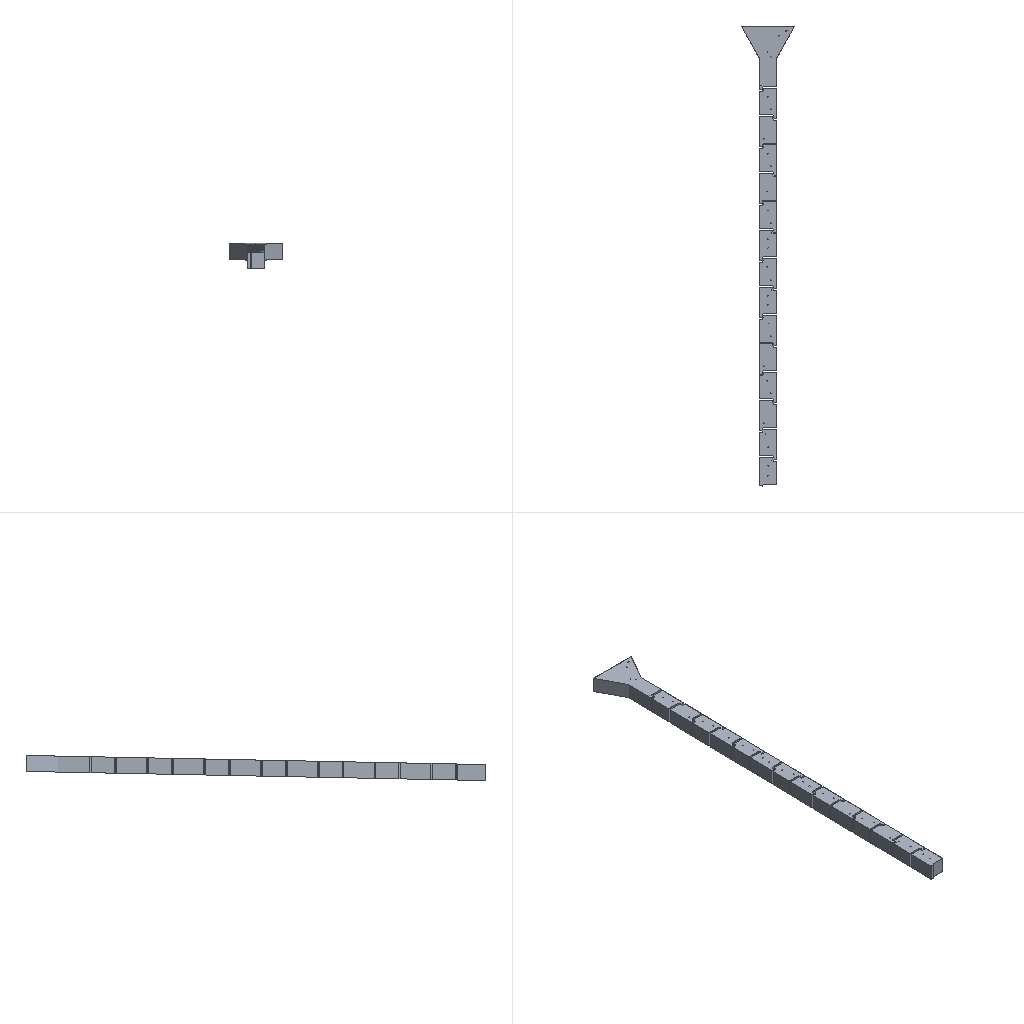Simulation study | ansys fluent
Set-up summary:
category,name,step,type,value,unit,region
solver,ansys_fluent,,Fluent 26.1.0
units,SI m-kg-s (Fluent internal),,stated,boundary values in the units shown in brackets; results in listed units
analysis,deck.cas,,cfd steady,"dimension=3D; solver=3d, dp, pbns, vof, rngke (3d, double precision, pressure-based, VOF, RNG k-epsilon); source_case=.cas"
model,Space,deck.cas,,3D
model,Time,deck.cas,,Steady
model,Viscous,deck.cas,,RNG k-epsilon turbulence model
model,Wall Treatment,deck.cas,,Standard Wall Functions
model,Heat Transfer,deck.cas,,Disabled
model,Multiphase,deck.cas,,Volume of Fluid
mesh,nodes,,,219317
mesh,elements,,,193302
mesh,faces,,,605099
cell_zone,part_1 (mixture),deck.cas,fluid,material=water-liquid,,zone 3
cell_zone,part_1 (air),deck.cas,fluid,material=air,,zone 3
cell_zone,part_1 (water),deck.cas,fluid,material=water-liquid,,zone 3
material,water-liquid (fluid),,Density,998.2,kg/m^3
material,water-liquid (fluid),,Viscosity,0.001003,kg/(m s)
material,air (fluid),,Density,1.225,kg/m^3
material,air (fluid),,Viscosity,1.7894e-05,kg/(m s)
material,aluminum (solid),,Density,2719,kg/m^3
bc,out1 (mixture),deck.cas,pressure-outlet,Backflow Direction Specification Method=Normal to Boundary,,zone 7
bc,out1 (air),deck.cas,pressure-outlet,,,zone 7
bc,out1 (water),deck.cas,pressure-outlet,,,zone 7
bc,int (mixture),deck.cas,velocity-inlet,Velocity Magnitude [m/s]=0.05,,zone 6
bc,int (air),deck.cas,velocity-inlet,,,zone 6
bc,int (water),deck.cas,velocity-inlet,Volume Fraction=1,,zone 6
bc,wall-part_1 (mixture),deck.cas,wall,Wall Motion=Stationary Wall; Shear Boundary Condition=No Slip,,zone 1
bc,wall-part_1 (air),deck.cas,wall,,,zone 1
bc,wall-part_1 (water),deck.cas,wall,,,zone 1
bc,wall (mixture),deck.cas,wall,Wall Motion=Stationary Wall; Shear Boundary Condition=No Slip,,zone 8
bc,wall (air),deck.cas,wall,,,zone 8
bc,wall (water),deck.cas,wall,,,zone 8
bc,out (mixture),deck.cas,pressure-outlet,Backflow Direction Specification Method=Normal to Boundary,,zone 9
bc,out (air),deck.cas,pressure-outlet,,,zone 9
bc,out (water),deck.cas,pressure-outlet,,,zone 9
Results summary:
result,mass flow rate int,deck.cas,,539.028,kg/s
result,mass flow rate out,deck.cas,,-135.762,kg/s
result,mass flow rate out1,deck.cas,,-205.751,kg/s
result,mass flow rate wall,deck.cas,,-0,kg/s
result,mass flow rate wall-part_1,deck.cas,,-0,kg/s
result,mass flow rate Net,deck.cas,,197.516,kg/s
result,wall force total wall,deck.cas,,"(-34.875, -3975.46, -667591)",N
result,wall force pressure wall,deck.cas,,"(-34.036, -3933.35, -667591)",N
result,wall force viscous wall,deck.cas,,"(-0.8381, -42.114, 0.5023)",N
result,wall force total wall-part_1,deck.cas,,"(108.811, -19370.5, -0.4062)",N
result,wall force pressure wall-part_1,deck.cas,,"(109.131, -19358.2, 0)",N
result,wall force viscous wall-part_1,deck.cas,,"(-0.3197, -12.311, -0.4062)",N
result,wall force total Net,deck.cas,,"(73.936, -23346, -667591)",N
result,wall force pressure Net,deck.cas,,"(75.094, -23291.5, -667591)",N
result,wall force viscous Net,deck.cas,,"(-1.158, -54.425, 0.09609)",N